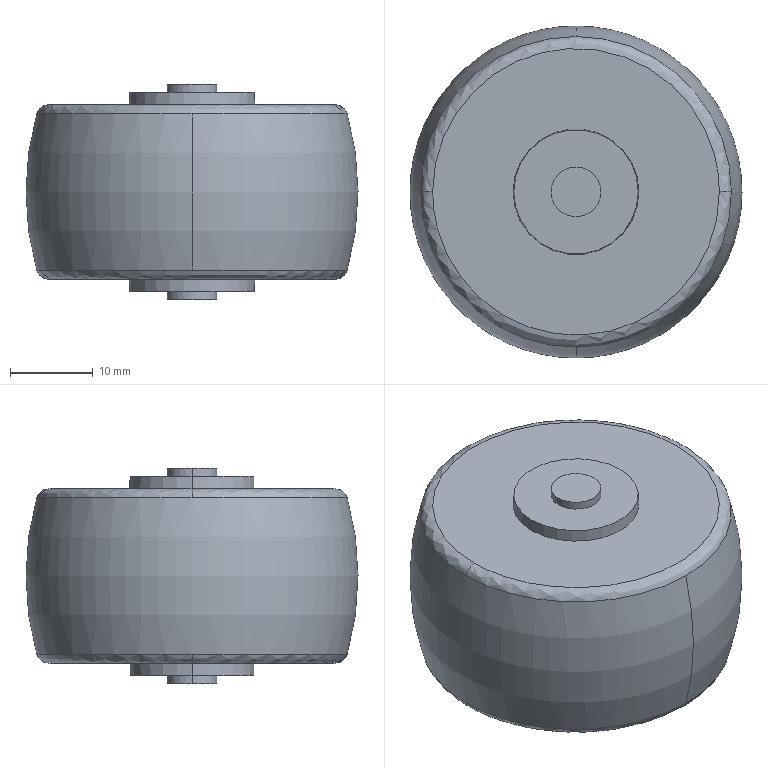Part | STEP file | _CMAZ40-N_w | 1 solid | 20 faces | box 40 x 40 x 26 mm | volume 25557 mm3 | plane 6 | spline 4 | cone 4 | cylinder 4 | torus 2 | commonest cylinder face diameters 6 x4
STEP:
#1=CARTESIAN_POINT('',(-17.268,0.,-10.5));
#2=VERTEX_POINT('',#1);
#3=CARTESIAN_POINT('',(17.268,0.,-10.5));
#4=VERTEX_POINT('',#3);
#5=CARTESIAN_POINT('',(-17.268,0.,-10.5));
#6=CARTESIAN_POINT('',(-17.268,-34.537,-10.5));
#7=CARTESIAN_POINT('',(17.268,-34.537,-10.5));
#8=CARTESIAN_POINT('',(17.268,0.,-10.5));
#9=(BOUNDED_CURVE()B_SPLINE_CURVE(3,(#5,#6,#7,#8),.UNSPECIFIED.,.F.,.T.)B_SPLINE_CURVE_WITH_KNOTS((4,4),(0.,0.5),.UNSPECIFIED.)CURVE()GEOMETRIC_REPRESENTATION_ITEM()RATIONAL_B_SPLINE_CURVE((1.,0.3333,0.3333,1.))REPRESENTATION_ITEM(''));
#10=EDGE_CURVE('',#2,#4,#9,.T.);
#11=ORIENTED_EDGE('',*,*,#10,.T.);
#12=CARTESIAN_POINT('',(18.713,0.,-9.403));
#13=VERTEX_POINT('',#12);
#14=CARTESIAN_POINT('',(17.268,0.,-9.));
#15=DIRECTION('',(0.,-1.,0.));
#16=DIRECTION('',(1.,0.,0.));
#17=AXIS2_PLACEMENT_3D('',#14,#15,#16);
#18=CIRCLE('',#17,1.5);
#19=EDGE_CURVE('',#4,#13,#18,.T.);
#20=ORIENTED_EDGE('',*,*,#19,.T.);
#21=CARTESIAN_POINT('',(0.,-18.713,-9.403));
#22=VERTEX_POINT('',#21);
#23=CARTESIAN_POINT('',(0.,0.,-9.403));
#24=DIRECTION('',(0.,0.,1.));
#25=DIRECTION('',(0.,-1.,0.));
#26=AXIS2_PLACEMENT_3D('',#23,#24,#25);
#27=CIRCLE('',#26,18.713);
#28=EDGE_CURVE('',#22,#13,#27,.T.);
#29=ORIENTED_EDGE('',*,*,#28,.F.);
#30=CARTESIAN_POINT('',(-18.713,0.,-9.403));
#31=VERTEX_POINT('',#30);
#32=CARTESIAN_POINT('',(0.,0.,-9.403));
#33=DIRECTION('',(0.,0.,1.));
#34=DIRECTION('',(0.,-1.,0.));
#35=AXIS2_PLACEMENT_3D('',#32,#33,#34);
#36=CIRCLE('',#35,18.713);
#37=EDGE_CURVE('',#31,#22,#36,.T.);
#38=ORIENTED_EDGE('',*,*,#37,.F.);
#39=CARTESIAN_POINT('',(-17.268,0.,-9.));
#40=DIRECTION('',(0.,1.,0.));
#41=DIRECTION('',(-1.,0.,0.));
#42=AXIS2_PLACEMENT_3D('',#39,#40,#41);
#43=CIRCLE('',#42,1.5);
#44=EDGE_CURVE('',#2,#31,#43,.T.);
#45=ORIENTED_EDGE('',*,*,#44,.F.);
#46=EDGE_LOOP('',(#11,#20,#29,#38,#45));
#47=FACE_OUTER_BOUND('',#46,.T.);
#48=CARTESIAN_POINT('',(17.268,0.,-10.5));
#49=CARTESIAN_POINT('',(17.268,-34.537,-10.5));
#50=CARTESIAN_POINT('',(-17.268,-34.537,-10.5));
#51=CARTESIAN_POINT('',(-17.268,0.,-10.5));
#52=CARTESIAN_POINT('',(17.968,0.,-10.5));
#53=CARTESIAN_POINT('',(17.968,-35.936,-10.5));
#54=CARTESIAN_POINT('',(-17.968,-35.936,-10.5));
#55=CARTESIAN_POINT('',(-17.968,0.,-10.5));
#56=CARTESIAN_POINT('',(18.525,0.,-10.077));
#57=CARTESIAN_POINT('',(18.525,-37.051,-10.077));
#58=CARTESIAN_POINT('',(-18.525,-37.051,-10.077));
#59=CARTESIAN_POINT('',(-18.525,0.,-10.077));
#60=CARTESIAN_POINT('',(18.713,0.,-9.403));
#61=CARTESIAN_POINT('',(18.713,-37.427,-9.403));
#62=CARTESIAN_POINT('',(-18.713,-37.427,-9.403));
#63=CARTESIAN_POINT('',(-18.713,0.,-9.403));
#64=(BOUNDED_SURFACE()B_SPLINE_SURFACE(3,3,((#48,#49,#50,#51),(#52,#53,#54,#55),(#56,#57,#58,#59),(#60,#61,#62,#63)),.UNSPECIFIED.,.F.,.F.,.T.)B_SPLINE_SURFACE_WITH_KNOTS((4,4),(4,4),(0.,1.),(0.,1.),.UNSPECIFIED.)GEOMETRIC_REPRESENTATION_ITEM()RATIONAL_B_SPLINE_SURFACE(((1.,0.3333,0.3333,1.),(0.8643,0.2881,0.2881,0.8643),(0.8643,0.2881,0.2881,0.8643),(1.,0.3333,0.3333,1.)))REPRESENTATION_ITEM('')SURFACE());
#65=ADVANCED_FACE('',(#47),#64,.T.);
#66=CARTESIAN_POINT('',(18.713,0.,9.403));
#67=VERTEX_POINT('',#66);
#68=CARTESIAN_POINT('',(0.,-18.713,9.403));
#69=VERTEX_POINT('',#68);
#70=CARTESIAN_POINT('',(0.,0.,9.403));
#71=DIRECTION('',(0.,0.,-1.));
#72=DIRECTION('',(-1.,0.,0.));
#73=AXIS2_PLACEMENT_3D('',#70,#71,#72);
#74=CIRCLE('',#73,18.713);
#75=EDGE_CURVE('',#67,#69,#74,.T.);
#76=ORIENTED_EDGE('',*,*,#75,.F.);
#77=CARTESIAN_POINT('',(17.268,0.,10.5));
#78=VERTEX_POINT('',#77);
#79=CARTESIAN_POINT('',(17.268,0.,9.));
#80=DIRECTION('',(0.,-1.,0.));
#81=DIRECTION('',(1.,0.,0.));
#82=AXIS2_PLACEMENT_3D('',#79,#80,#81);
#83=CIRCLE('',#82,1.5);
#84=EDGE_CURVE('',#67,#78,#83,.T.);
#85=ORIENTED_EDGE('',*,*,#84,.T.);
#86=CARTESIAN_POINT('',(-17.268,0.,10.5));
#87=VERTEX_POINT('',#86);
#88=CARTESIAN_POINT('',(17.268,0.,10.5));
#89=CARTESIAN_POINT('',(17.268,-34.537,10.5));
#90=CARTESIAN_POINT('',(-17.268,-34.537,10.5));
#91=CARTESIAN_POINT('',(-17.268,0.,10.5));
#92=(BOUNDED_CURVE()B_SPLINE_CURVE(3,(#88,#89,#90,#91),.UNSPECIFIED.,.F.,.F.)B_SPLINE_CURVE_WITH_KNOTS((4,4),(0.5,1.),.UNSPECIFIED.)CURVE()GEOMETRIC_REPRESENTATION_ITEM()RATIONAL_B_SPLINE_CURVE((1.,0.3333,0.3333,1.))REPRESENTATION_ITEM(''));
#93=EDGE_CURVE('',#78,#87,#92,.T.);
#94=ORIENTED_EDGE('',*,*,#93,.T.);
#95=CARTESIAN_POINT('',(-18.713,0.,9.403));
#96=VERTEX_POINT('',#95);
#97=CARTESIAN_POINT('',(-17.268,0.,9.));
#98=DIRECTION('',(0.,1.,0.));
#99=DIRECTION('',(-1.,0.,0.));
#100=AXIS2_PLACEMENT_3D('',#97,#98,#99);
#101=CIRCLE('',#100,1.5);
#102=EDGE_CURVE('',#96,#87,#101,.T.);
#103=ORIENTED_EDGE('',*,*,#102,.F.);
#104=CARTESIAN_POINT('',(0.,0.,9.403));
#105=DIRECTION('',(0.,0.,-1.));
#106=DIRECTION('',(-1.,0.,0.));
#107=AXIS2_PLACEMENT_3D('',#104,#105,#106);
#108=CIRCLE('',#107,18.713);
#109=EDGE_CURVE('',#69,#96,#108,.T.);
#110=ORIENTED_EDGE('',*,*,#109,.F.);
#111=EDGE_LOOP('',(#76,#85,#94,#103,#110));
#112=FACE_OUTER_BOUND('',#111,.T.);
#113=CARTESIAN_POINT('',(18.713,0.,9.403));
#114=CARTESIAN_POINT('',(18.713,-37.427,9.403));
#115=CARTESIAN_POINT('',(-18.713,-37.427,9.403));
#116=CARTESIAN_POINT('',(-18.713,0.,9.403));
#117=CARTESIAN_POINT('',(18.525,0.,10.077));
#118=CARTESIAN_POINT('',(18.525,-37.051,10.077));
#119=CARTESIAN_POINT('',(-18.525,-37.051,10.077));
#120=CARTESIAN_POINT('',(-18.525,0.,10.077));
#121=CARTESIAN_POINT('',(17.968,0.,10.5));
#122=CARTESIAN_POINT('',(17.968,-35.936,10.5));
#123=CARTESIAN_POINT('',(-17.968,-35.936,10.5));
#124=CARTESIAN_POINT('',(-17.968,0.,10.5));
#125=CARTESIAN_POINT('',(17.268,0.,10.5));
#126=CARTESIAN_POINT('',(17.268,-34.537,10.5));
#127=CARTESIAN_POINT('',(-17.268,-34.537,10.5));
#128=CARTESIAN_POINT('',(-17.268,0.,10.5));
#129=(BOUNDED_SURFACE()B_SPLINE_SURFACE(3,3,((#113,#114,#115,#116),(#117,#118,#119,#120),(#121,#122,#123,#124),(#125,#126,#127,#128)),.UNSPECIFIED.,.F.,.F.,.F.)B_SPLINE_SURFACE_WITH_KNOTS((4,4),(4,4),(0.,1.),(0.,1.),.UNSPECIFIED.)GEOMETRIC_REPRESENTATION_ITEM()RATIONAL_B_SPLINE_SURFACE(((1.,0.3333,0.3333,1.),(0.8643,0.2881,0.2881,0.8643),(0.8643,0.2881,0.2881,0.8643),(1.,0.3333,0.3333,1.)))REPRESENTATION_ITEM('')SURFACE());
#130=ADVANCED_FACE('',(#112),#129,.T.);
#131=CARTESIAN_POINT('',(0.,18.713,9.403));
#132=VERTEX_POINT('',#131);
#133=CARTESIAN_POINT('',(0.,0.,9.403));
#134=DIRECTION('',(0.,0.,-1.));
#135=DIRECTION('',(-1.,0.,0.));
#136=AXIS2_PLACEMENT_3D('',#133,#134,#135);
#137=CIRCLE('',#136,18.713);
#138=EDGE_CURVE('',#132,#67,#137,.T.);
#139=ORIENTED_EDGE('',*,*,#138,.T.);
#140=ORIENTED_EDGE('',*,*,#75,.T.);
#141=CARTESIAN_POINT('',(0.,15.,0.));
#142=DIRECTION('',(1.,0.,0.));
#143=DIRECTION('',(0.,1.,0.));
#144=AXIS2_PLACEMENT_3D('',#141,#142,#143);
#145=CIRCLE('',#144,35.);
#146=EDGE_CURVE('',#69,#22,#145,.T.);
#147=ORIENTED_EDGE('',*,*,#146,.T.);
#148=ORIENTED_EDGE('',*,*,#28,.T.);
#149=CARTESIAN_POINT('',(0.,18.713,-9.403));
#150=VERTEX_POINT('',#149);
#151=CARTESIAN_POINT('',(0.,0.,-9.403));
#152=DIRECTION('',(0.,0.,1.));
#153=DIRECTION('',(0.,-1.,0.));
#154=AXIS2_PLACEMENT_3D('',#151,#152,#153);
#155=CIRCLE('',#154,18.713);
#156=EDGE_CURVE('',#13,#150,#155,.T.);
#157=ORIENTED_EDGE('',*,*,#156,.T.);
#158=CARTESIAN_POINT('',(0.,-15.,0.));
#159=DIRECTION('',(-1.,0.,0.));
#160=DIRECTION('',(0.,0.,1.));
#161=AXIS2_PLACEMENT_3D('',#158,#159,#160);
#162=CIRCLE('',#161,35.);
#163=EDGE_CURVE('',#132,#150,#162,.T.);
#164=ORIENTED_EDGE('',*,*,#163,.F.);
#165=EDGE_LOOP('',(#139,#140,#147,#148,#157,#164));
#166=FACE_OUTER_BOUND('',#165,.T.);
#167=CARTESIAN_POINT('',(0.,0.,0.));
#168=DIRECTION('',(0.,0.,-1.));
#169=DIRECTION('',(0.,1.,0.));
#170=AXIS2_PLACEMENT_3D('',#167,#168,#169);
#171=TOROIDAL_SURFACE('',#170,-15.,35.);
#172=ADVANCED_FACE('',(#166),#171,.T.);
#173=CARTESIAN_POINT('',(7.5,0.,-12.));
#174=VERTEX_POINT('',#173);
#175=CARTESIAN_POINT('',(-7.5,0.,-12.));
#176=VERTEX_POINT('',#175);
#177=CARTESIAN_POINT('',(0.,0.,-12.));
#178=DIRECTION('',(0.,0.,1.));
#179=DIRECTION('',(1.,0.,0.));
#180=AXIS2_PLACEMENT_3D('',#177,#178,#179);
#181=CIRCLE('',#180,7.5);
#182=EDGE_CURVE('',#174,#176,#181,.T.);
#183=ORIENTED_EDGE('',*,*,#182,.T.);
#184=CARTESIAN_POINT('',(-7.579,0.,-10.5));
#185=VERTEX_POINT('',#184);
#186=CARTESIAN_POINT('',(-7.579,0.,-10.5));
#187=DIRECTION('',(-0.05226,0.,0.9986));
#188=VECTOR('',#187,1000.);
#189=LINE('',#186,#188);
#190=EDGE_CURVE('',#176,#185,#189,.T.);
#191=ORIENTED_EDGE('',*,*,#190,.T.);
#192=CARTESIAN_POINT('',(7.579,0.,-10.5));
#193=VERTEX_POINT('',#192);
#194=CARTESIAN_POINT('',(0.,0.,-10.5));
#195=DIRECTION('',(0.,0.,-1.));
#196=DIRECTION('',(1.,0.,0.));
#197=AXIS2_PLACEMENT_3D('',#194,#195,#196);
#198=CIRCLE('',#197,7.579);
#199=EDGE_CURVE('',#185,#193,#198,.T.);
#200=ORIENTED_EDGE('',*,*,#199,.T.);
#201=CARTESIAN_POINT('',(7.579,0.,-10.5));
#202=DIRECTION('',(0.05226,0.,0.9986));
#203=VECTOR('',#202,1000.);
#204=LINE('',#201,#203);
#205=EDGE_CURVE('',#174,#193,#204,.T.);
#206=ORIENTED_EDGE('',*,*,#205,.F.);
#207=EDGE_LOOP('',(#183,#191,#200,#206));
#208=FACE_OUTER_BOUND('',#207,.T.);
#209=CARTESIAN_POINT('',(0.,0.,-10.5));
#210=DIRECTION('',(0.,0.,1.));
#211=DIRECTION('',(1.,0.,0.));
#212=AXIS2_PLACEMENT_3D('',#209,#210,#211);
#213=CONICAL_SURFACE('',#212,7.579,0.05229);
#214=ADVANCED_FACE('',(#208),#213,.T.);
#215=CARTESIAN_POINT('',(-7.5,0.,12.));
#216=VERTEX_POINT('',#215);
#217=CARTESIAN_POINT('',(7.5,0.,12.));
#218=VERTEX_POINT('',#217);
#219=CARTESIAN_POINT('',(0.,0.,12.));
#220=DIRECTION('',(0.,0.,-1.));
#221=DIRECTION('',(-1.,0.,0.));
#222=AXIS2_PLACEMENT_3D('',#219,#220,#221);
#223=CIRCLE('',#222,7.5);
#224=EDGE_CURVE('',#216,#218,#223,.T.);
#225=ORIENTED_EDGE('',*,*,#224,.T.);
#226=CARTESIAN_POINT('',(7.579,0.,10.5));
#227=VERTEX_POINT('',#226);
#228=CARTESIAN_POINT('',(7.579,0.,10.5));
#229=DIRECTION('',(0.05226,0.,-0.9986));
#230=VECTOR('',#229,1000.);
#231=LINE('',#228,#230);
#232=EDGE_CURVE('',#218,#227,#231,.T.);
#233=ORIENTED_EDGE('',*,*,#232,.T.);
#234=CARTESIAN_POINT('',(-7.579,0.,10.5));
#235=VERTEX_POINT('',#234);
#236=CARTESIAN_POINT('',(0.,0.,10.5));
#237=DIRECTION('',(0.,0.,1.));
#238=DIRECTION('',(-1.,0.,0.));
#239=AXIS2_PLACEMENT_3D('',#236,#237,#238);
#240=CIRCLE('',#239,7.579);
#241=EDGE_CURVE('',#227,#235,#240,.T.);
#242=ORIENTED_EDGE('',*,*,#241,.T.);
#243=CARTESIAN_POINT('',(-7.579,0.,10.5));
#244=DIRECTION('',(-0.05226,0.,-0.9986));
#245=VECTOR('',#244,1000.);
#246=LINE('',#243,#245);
#247=EDGE_CURVE('',#216,#235,#246,.T.);
#248=ORIENTED_EDGE('',*,*,#247,.F.);
#249=EDGE_LOOP('',(#225,#233,#242,#248));
#250=FACE_OUTER_BOUND('',#249,.T.);
#251=CARTESIAN_POINT('',(0.,0.,10.5));
#252=DIRECTION('',(0.,0.,-1.));
#253=DIRECTION('',(-1.,0.,0.));
#254=AXIS2_PLACEMENT_3D('',#251,#252,#253);
#255=CONICAL_SURFACE('',#254,7.579,0.05229);
#256=ADVANCED_FACE('',(#250),#255,.T.);
#257=CARTESIAN_POINT('',(3.,0.,-13.));
#258=VERTEX_POINT('',#257);
#259=CARTESIAN_POINT('',(-3.,0.,-13.));
#260=VERTEX_POINT('',#259);
#261=CARTESIAN_POINT('',(0.,0.,-13.));
#262=DIRECTION('',(0.,0.,1.));
#263=DIRECTION('',(1.,0.,0.));
#264=AXIS2_PLACEMENT_3D('',#261,#262,#263);
#265=CIRCLE('',#264,3.);
#266=EDGE_CURVE('',#258,#260,#265,.T.);
#267=ORIENTED_EDGE('',*,*,#266,.T.);
#268=CARTESIAN_POINT('',(-3.,0.,-12.));
#269=VERTEX_POINT('',#268);
#270=CARTESIAN_POINT('',(-3.,0.,-13.));
#271=DIRECTION('',(0.,0.,1.));
#272=VECTOR('',#271,1000.);
#273=LINE('',#270,#272);
#274=EDGE_CURVE('',#260,#269,#273,.T.);
#275=ORIENTED_EDGE('',*,*,#274,.T.);
#276=CARTESIAN_POINT('',(3.,0.,-12.));
#277=VERTEX_POINT('',#276);
#278=CARTESIAN_POINT('',(0.,0.,-12.));
#279=DIRECTION('',(0.,0.,-1.));
#280=DIRECTION('',(1.,0.,0.));
#281=AXIS2_PLACEMENT_3D('',#278,#279,#280);
#282=CIRCLE('',#281,3.);
#283=EDGE_CURVE('',#269,#277,#282,.T.);
#284=ORIENTED_EDGE('',*,*,#283,.T.);
#285=CARTESIAN_POINT('',(3.,0.,-13.));
#286=DIRECTION('',(0.,0.,1.));
#287=VECTOR('',#286,1000.);
#288=LINE('',#285,#287);
#289=EDGE_CURVE('',#258,#277,#288,.T.);
#290=ORIENTED_EDGE('',*,*,#289,.F.);
#291=EDGE_LOOP('',(#267,#275,#284,#290));
#292=FACE_OUTER_BOUND('',#291,.T.);
#293=CARTESIAN_POINT('',(0.,0.,-13.));
#294=DIRECTION('',(0.,0.,1.));
#295=DIRECTION('',(1.,0.,0.));
#296=AXIS2_PLACEMENT_3D('',#293,#294,#295);
#297=CYLINDRICAL_SURFACE('',#296,3.);
#298=ADVANCED_FACE('',(#292),#297,.T.);
#299=CARTESIAN_POINT('',(3.,0.,12.));
#300=VERTEX_POINT('',#299);
#301=CARTESIAN_POINT('',(-3.,0.,12.));
#302=VERTEX_POINT('',#301);
#303=CARTESIAN_POINT('',(0.,0.,12.));
#304=DIRECTION('',(0.,0.,1.));
#305=DIRECTION('',(1.,0.,0.));
#306=AXIS2_PLACEMENT_3D('',#303,#304,#305);
#307=CIRCLE('',#306,3.);
#308=EDGE_CURVE('',#300,#302,#307,.T.);
#309=ORIENTED_EDGE('',*,*,#308,.T.);
#310=CARTESIAN_POINT('',(-3.,0.,13.));
#311=VERTEX_POINT('',#310);
#312=CARTESIAN_POINT('',(-3.,0.,-13.));
#313=DIRECTION('',(0.,0.,1.));
#314=VECTOR('',#313,1000.);
#315=LINE('',#312,#314);
#316=EDGE_CURVE('',#302,#311,#315,.T.);
#317=ORIENTED_EDGE('',*,*,#316,.T.);
#318=CARTESIAN_POINT('',(3.,0.,13.));
#319=VERTEX_POINT('',#318);
#320=CARTESIAN_POINT('',(0.,0.,13.));
#321=DIRECTION('',(0.,0.,-1.));
#322=DIRECTION('',(1.,0.,0.));
#323=AXIS2_PLACEMENT_3D('',#320,#321,#322);
#324=CIRCLE('',#323,3.);
#325=EDGE_CURVE('',#311,#319,#324,.T.);
#326=ORIENTED_EDGE('',*,*,#325,.T.);
#327=CARTESIAN_POINT('',(3.,0.,-13.));
#328=DIRECTION('',(0.,0.,1.));
#329=VECTOR('',#328,1000.);
#330=LINE('',#327,#329);
#331=EDGE_CURVE('',#300,#319,#330,.T.);
#332=ORIENTED_EDGE('',*,*,#331,.F.);
#333=EDGE_LOOP('',(#309,#317,#326,#332));
#334=FACE_OUTER_BOUND('',#333,.T.);
#335=CARTESIAN_POINT('',(0.,0.,-13.));
#336=DIRECTION('',(0.,0.,1.));
#337=DIRECTION('',(1.,0.,0.));
#338=AXIS2_PLACEMENT_3D('',#335,#336,#337);
#339=CYLINDRICAL_SURFACE('',#338,3.);
#340=ADVANCED_FACE('',(#334),#339,.T.);
#341=ORIENTED_EDGE('',*,*,#146,.F.);
#342=ORIENTED_EDGE('',*,*,#109,.T.);
#343=CARTESIAN_POINT('',(0.,0.,9.403));
#344=DIRECTION('',(0.,0.,-1.));
#345=DIRECTION('',(-1.,0.,0.));
#346=AXIS2_PLACEMENT_3D('',#343,#344,#345);
#347=CIRCLE('',#346,18.713);
#348=EDGE_CURVE('',#96,#132,#347,.T.);
#349=ORIENTED_EDGE('',*,*,#348,.T.);
#350=ORIENTED_EDGE('',*,*,#163,.T.);
#351=CARTESIAN_POINT('',(0.,0.,-9.403));
#352=DIRECTION('',(0.,0.,1.));
#353=DIRECTION('',(0.,-1.,0.));
#354=AXIS2_PLACEMENT_3D('',#351,#352,#353);
#355=CIRCLE('',#354,18.713);
#356=EDGE_CURVE('',#150,#31,#355,.T.);
#357=ORIENTED_EDGE('',*,*,#356,.T.);
#358=ORIENTED_EDGE('',*,*,#37,.T.);
#359=EDGE_LOOP('',(#341,#342,#349,#350,#357,#358));
#360=FACE_OUTER_BOUND('',#359,.T.);
#361=CARTESIAN_POINT('',(0.,0.,0.));
#362=DIRECTION('',(0.,0.,-1.));
#363=DIRECTION('',(0.,1.,0.));
#364=AXIS2_PLACEMENT_3D('',#361,#362,#363);
#365=TOROIDAL_SURFACE('',#364,-15.,35.);
#366=ADVANCED_FACE('',(#360),#365,.T.);
#367=ORIENTED_EDGE('',*,*,#19,.F.);
#368=CARTESIAN_POINT('',(17.268,0.,-10.5));
#369=CARTESIAN_POINT('',(17.268,34.537,-10.5));
#370=CARTESIAN_POINT('',(-17.268,34.537,-10.5));
#371=CARTESIAN_POINT('',(-17.268,0.,-10.5));
#372=(BOUNDED_CURVE()B_SPLINE_CURVE(3,(#368,#369,#370,#371),.UNSPECIFIED.,.F.,.T.)B_SPLINE_CURVE_WITH_KNOTS((4,4),(0.5,1.),.UNSPECIFIED.)CURVE()GEOMETRIC_REPRESENTATION_ITEM()RATIONAL_B_SPLINE_CURVE((1.,0.3333,0.3333,1.))REPRESENTATION_ITEM(''));
#373=EDGE_CURVE('',#4,#2,#372,.T.);
#374=ORIENTED_EDGE('',*,*,#373,.T.);
#375=ORIENTED_EDGE('',*,*,#44,.T.);
#376=ORIENTED_EDGE('',*,*,#356,.F.);
#377=ORIENTED_EDGE('',*,*,#156,.F.);
#378=EDGE_LOOP('',(#367,#374,#375,#376,#377));
#379=FACE_OUTER_BOUND('',#378,.T.);
#380=CARTESIAN_POINT('',(-17.268,0.,-10.5));
#381=CARTESIAN_POINT('',(-17.268,34.537,-10.5));
#382=CARTESIAN_POINT('',(17.268,34.537,-10.5));
#383=CARTESIAN_POINT('',(17.268,0.,-10.5));
#384=CARTESIAN_POINT('',(-17.968,0.,-10.5));
#385=CARTESIAN_POINT('',(-17.968,35.936,-10.5));
#386=CARTESIAN_POINT('',(17.968,35.936,-10.5));
#387=CARTESIAN_POINT('',(17.968,0.,-10.5));
#388=CARTESIAN_POINT('',(-18.525,0.,-10.077));
#389=CARTESIAN_POINT('',(-18.525,37.051,-10.077));
#390=CARTESIAN_POINT('',(18.525,37.051,-10.077));
#391=CARTESIAN_POINT('',(18.525,0.,-10.077));
#392=CARTESIAN_POINT('',(-18.713,0.,-9.403));
#393=CARTESIAN_POINT('',(-18.713,37.427,-9.403));
#394=CARTESIAN_POINT('',(18.713,37.427,-9.403));
#395=CARTESIAN_POINT('',(18.713,0.,-9.403));
#396=(BOUNDED_SURFACE()B_SPLINE_SURFACE(3,3,((#380,#381,#382,#383),(#384,#385,#386,#387),(#388,#389,#390,#391),(#392,#393,#394,#395)),.UNSPECIFIED.,.F.,.F.,.F.)B_SPLINE_SURFACE_WITH_KNOTS((4,4),(4,4),(0.,1.),(0.,1.),.UNSPECIFIED.)GEOMETRIC_REPRESENTATION_ITEM()RATIONAL_B_SPLINE_SURFACE(((1.,0.3333,0.3333,1.),(0.8643,0.2881,0.2881,0.8643),(0.8643,0.2881,0.2881,0.8643),(1.,0.3333,0.3333,1.)))REPRESENTATION_ITEM('')SURFACE());
#397=ADVANCED_FACE('',(#379),#396,.T.);
#398=ORIENTED_EDGE('',*,*,#84,.F.);
#399=ORIENTED_EDGE('',*,*,#138,.F.);
#400=ORIENTED_EDGE('',*,*,#348,.F.);
#401=ORIENTED_EDGE('',*,*,#102,.T.);
#402=CARTESIAN_POINT('',(-17.268,0.,10.5));
#403=CARTESIAN_POINT('',(-17.268,34.537,10.5));
#404=CARTESIAN_POINT('',(17.268,34.537,10.5));
#405=CARTESIAN_POINT('',(17.268,0.,10.5));
#406=(BOUNDED_CURVE()B_SPLINE_CURVE(3,(#402,#403,#404,#405),.UNSPECIFIED.,.F.,.T.)B_SPLINE_CURVE_WITH_KNOTS((4,4),(0.,0.5),.UNSPECIFIED.)CURVE()GEOMETRIC_REPRESENTATION_ITEM()RATIONAL_B_SPLINE_CURVE((1.,0.3333,0.3333,1.))REPRESENTATION_ITEM(''));
#407=EDGE_CURVE('',#87,#78,#406,.T.);
#408=ORIENTED_EDGE('',*,*,#407,.T.);
#409=EDGE_LOOP('',(#398,#399,#400,#401,#408));
#410=FACE_OUTER_BOUND('',#409,.T.);
#411=CARTESIAN_POINT('',(-18.713,0.,9.403));
#412=CARTESIAN_POINT('',(-18.713,37.427,9.403));
#413=CARTESIAN_POINT('',(18.713,37.427,9.403));
#414=CARTESIAN_POINT('',(18.713,0.,9.403));
#415=CARTESIAN_POINT('',(-18.525,0.,10.077));
#416=CARTESIAN_POINT('',(-18.525,37.051,10.077));
#417=CARTESIAN_POINT('',(18.525,37.051,10.077));
#418=CARTESIAN_POINT('',(18.525,0.,10.077));
#419=CARTESIAN_POINT('',(-17.968,0.,10.5));
#420=CARTESIAN_POINT('',(-17.968,35.936,10.5));
#421=CARTESIAN_POINT('',(17.968,35.936,10.5));
#422=CARTESIAN_POINT('',(17.968,0.,10.5));
#423=CARTESIAN_POINT('',(-17.268,0.,10.5));
#424=CARTESIAN_POINT('',(-17.268,34.537,10.5));
#425=CARTESIAN_POINT('',(17.268,34.537,10.5));
#426=CARTESIAN_POINT('',(17.268,0.,10.5));
#427=(BOUNDED_SURFACE()B_SPLINE_SURFACE(3,3,((#411,#412,#413,#414),(#415,#416,#417,#418),(#419,#420,#421,#422),(#423,#424,#425,#426)),.UNSPECIFIED.,.F.,.F.,.F.)B_SPLINE_SURFACE_WITH_KNOTS((4,4),(4,4),(0.,1.),(0.,1.),.UNSPECIFIED.)GEOMETRIC_REPRESENTATION_ITEM()RATIONAL_B_SPLINE_SURFACE(((1.,0.3333,0.3333,1.),(0.8643,0.2881,0.2881,0.8643),(0.8643,0.2881,0.2881,0.8643),(1.,0.3333,0.3333,1.)))REPRESENTATION_ITEM('')SURFACE());
#428=ADVANCED_FACE('',(#410),#427,.T.);
#429=ORIENTED_EDGE('',*,*,#10,.F.);
#430=ORIENTED_EDGE('',*,*,#373,.F.);
#431=EDGE_LOOP('',(#429,#430));
#432=FACE_OUTER_BOUND('',#431,.T.);
#433=CARTESIAN_POINT('',(0.,0.,-10.5));
#434=DIRECTION('',(0.,0.,-1.));
#435=DIRECTION('',(1.,0.,0.));
#436=AXIS2_PLACEMENT_3D('',#433,#434,#435);
#437=CIRCLE('',#436,7.579);
#438=EDGE_CURVE('',#193,#185,#437,.T.);
#439=ORIENTED_EDGE('',*,*,#438,.F.);
#440=ORIENTED_EDGE('',*,*,#199,.F.);
#441=EDGE_LOOP('',(#439,#440));
#442=FACE_BOUND('',#441,.T.);
#443=CARTESIAN_POINT('',(0.,17.268,-10.5));
#444=DIRECTION('',(0.,0.,1.));
#445=DIRECTION('',(1.,0.,0.));
#446=AXIS2_PLACEMENT_3D('',#443,#444,#445);
#447=PLANE('',#446);
#448=ADVANCED_FACE('',(#432,#442),#447,.F.);
#449=CARTESIAN_POINT('',(0.,0.,10.5));
#450=DIRECTION('',(0.,0.,1.));
#451=DIRECTION('',(-1.,0.,0.));
#452=AXIS2_PLACEMENT_3D('',#449,#450,#451);
#453=CIRCLE('',#452,7.579);
#454=EDGE_CURVE('',#235,#227,#453,.T.);
#455=ORIENTED_EDGE('',*,*,#454,.F.);
#456=ORIENTED_EDGE('',*,*,#241,.F.);
#457=EDGE_LOOP('',(#455,#456));
#458=FACE_BOUND('',#457,.T.);
#459=ORIENTED_EDGE('',*,*,#407,.F.);
#460=ORIENTED_EDGE('',*,*,#93,.F.);
#461=EDGE_LOOP('',(#459,#460));
#462=FACE_OUTER_BOUND('',#461,.T.);
#463=CARTESIAN_POINT('',(0.,7.579,10.5));
#464=DIRECTION('',(0.,0.,-1.));
#465=DIRECTION('',(-1.,0.,0.));
#466=AXIS2_PLACEMENT_3D('',#463,#464,#465);
#467=PLANE('',#466);
#468=ADVANCED_FACE('',(#458,#462),#467,.F.);
#469=ORIENTED_EDGE('',*,*,#190,.F.);
#470=CARTESIAN_POINT('',(0.,0.,-12.));
#471=DIRECTION('',(0.,0.,1.));
#472=DIRECTION('',(1.,0.,0.));
#473=AXIS2_PLACEMENT_3D('',#470,#471,#472);
#474=CIRCLE('',#473,7.5);
#475=EDGE_CURVE('',#176,#174,#474,.T.);
#476=ORIENTED_EDGE('',*,*,#475,.T.);
#477=ORIENTED_EDGE('',*,*,#205,.T.);
#478=ORIENTED_EDGE('',*,*,#438,.T.);
#479=EDGE_LOOP('',(#469,#476,#477,#478));
#480=FACE_OUTER_BOUND('',#479,.T.);
#481=CARTESIAN_POINT('',(0.,0.,-10.5));
#482=DIRECTION('',(0.,0.,1.));
#483=DIRECTION('',(1.,0.,0.));
#484=AXIS2_PLACEMENT_3D('',#481,#482,#483);
#485=CONICAL_SURFACE('',#484,7.579,0.05229);
#486=ADVANCED_FACE('',(#480),#485,.T.);
#487=ORIENTED_EDGE('',*,*,#232,.F.);
#488=CARTESIAN_POINT('',(0.,0.,12.));
#489=DIRECTION('',(0.,0.,-1.));
#490=DIRECTION('',(-1.,0.,0.));
#491=AXIS2_PLACEMENT_3D('',#488,#489,#490);
#492=CIRCLE('',#491,7.5);
#493=EDGE_CURVE('',#218,#216,#492,.T.);
#494=ORIENTED_EDGE('',*,*,#493,.T.);
#495=ORIENTED_EDGE('',*,*,#247,.T.);
#496=ORIENTED_EDGE('',*,*,#454,.T.);
#497=EDGE_LOOP('',(#487,#494,#495,#496));
#498=FACE_OUTER_BOUND('',#497,.T.);
#499=CARTESIAN_POINT('',(0.,0.,10.5));
#500=DIRECTION('',(0.,0.,-1.));
#501=DIRECTION('',(-1.,0.,0.));
#502=AXIS2_PLACEMENT_3D('',#499,#500,#501);
#503=CONICAL_SURFACE('',#502,7.579,0.05229);
#504=ADVANCED_FACE('',(#498),#503,.T.);
#505=ORIENTED_EDGE('',*,*,#182,.F.);
#506=ORIENTED_EDGE('',*,*,#475,.F.);
#507=EDGE_LOOP('',(#505,#506));
#508=FACE_OUTER_BOUND('',#507,.T.);
#509=CARTESIAN_POINT('',(0.,0.,-12.));
#510=DIRECTION('',(0.,0.,-1.));
#511=DIRECTION('',(1.,0.,0.));
#512=AXIS2_PLACEMENT_3D('',#509,#510,#511);
#513=CIRCLE('',#512,3.);
#514=EDGE_CURVE('',#277,#269,#513,.T.);
#515=ORIENTED_EDGE('',*,*,#514,.F.);
#516=ORIENTED_EDGE('',*,*,#283,.F.);
#517=EDGE_LOOP('',(#515,#516));
#518=FACE_BOUND('',#517,.T.);
#519=CARTESIAN_POINT('',(0.,7.5,-12.));
#520=DIRECTION('',(0.,0.,1.));
#521=DIRECTION('',(1.,0.,0.));
#522=AXIS2_PLACEMENT_3D('',#519,#520,#521);
#523=PLANE('',#522);
#524=ADVANCED_FACE('',(#508,#518),#523,.F.);
#525=ORIENTED_EDGE('',*,*,#308,.F.);
#526=CARTESIAN_POINT('',(0.,0.,12.));
#527=DIRECTION('',(0.,0.,1.));
#528=DIRECTION('',(1.,0.,0.));
#529=AXIS2_PLACEMENT_3D('',#526,#527,#528);
#530=CIRCLE('',#529,3.);
#531=EDGE_CURVE('',#302,#300,#530,.T.);
#532=ORIENTED_EDGE('',*,*,#531,.F.);
#533=EDGE_LOOP('',(#525,#532));
#534=FACE_BOUND('',#533,.T.);
#535=ORIENTED_EDGE('',*,*,#224,.F.);
#536=ORIENTED_EDGE('',*,*,#493,.F.);
#537=EDGE_LOOP('',(#535,#536));
#538=FACE_OUTER_BOUND('',#537,.T.);
#539=CARTESIAN_POINT('',(0.,3.,12.));
#540=DIRECTION('',(0.,0.,-1.));
#541=DIRECTION('',(-1.,0.,0.));
#542=AXIS2_PLACEMENT_3D('',#539,#540,#541);
#543=PLANE('',#542);
#544=ADVANCED_FACE('',(#534,#538),#543,.F.);
#545=ORIENTED_EDGE('',*,*,#274,.F.);
#546=CARTESIAN_POINT('',(0.,0.,-13.));
#547=DIRECTION('',(0.,0.,1.));
#548=DIRECTION('',(1.,0.,0.));
#549=AXIS2_PLACEMENT_3D('',#546,#547,#548);
#550=CIRCLE('',#549,3.);
#551=EDGE_CURVE('',#260,#258,#550,.T.);
#552=ORIENTED_EDGE('',*,*,#551,.T.);
#553=ORIENTED_EDGE('',*,*,#289,.T.);
#554=ORIENTED_EDGE('',*,*,#514,.T.);
#555=EDGE_LOOP('',(#545,#552,#553,#554));
#556=FACE_OUTER_BOUND('',#555,.T.);
#557=CARTESIAN_POINT('',(0.,0.,-13.));
#558=DIRECTION('',(0.,0.,1.));
#559=DIRECTION('',(1.,0.,0.));
#560=AXIS2_PLACEMENT_3D('',#557,#558,#559);
#561=CYLINDRICAL_SURFACE('',#560,3.);
#562=ADVANCED_FACE('',(#556),#561,.T.);
#563=ORIENTED_EDGE('',*,*,#316,.F.);
#564=ORIENTED_EDGE('',*,*,#531,.T.);
#565=ORIENTED_EDGE('',*,*,#331,.T.);
#566=CARTESIAN_POINT('',(0.,0.,13.));
#567=DIRECTION('',(0.,0.,-1.));
#568=DIRECTION('',(1.,0.,0.));
#569=AXIS2_PLACEMENT_3D('',#566,#567,#568);
#570=CIRCLE('',#569,3.);
#571=EDGE_CURVE('',#319,#311,#570,.T.);
#572=ORIENTED_EDGE('',*,*,#571,.T.);
#573=EDGE_LOOP('',(#563,#564,#565,#572));
#574=FACE_OUTER_BOUND('',#573,.T.);
#575=CARTESIAN_POINT('',(0.,0.,-13.));
#576=DIRECTION('',(0.,0.,1.));
#577=DIRECTION('',(1.,0.,0.));
#578=AXIS2_PLACEMENT_3D('',#575,#576,#577);
#579=CYLINDRICAL_SURFACE('',#578,3.);
#580=ADVANCED_FACE('',(#574),#579,.T.);
#581=ORIENTED_EDGE('',*,*,#266,.F.);
#582=ORIENTED_EDGE('',*,*,#551,.F.);
#583=EDGE_LOOP('',(#581,#582));
#584=FACE_OUTER_BOUND('',#583,.T.);
#585=CARTESIAN_POINT('',(0.,3.,-13.));
#586=DIRECTION('',(0.,0.,1.));
#587=DIRECTION('',(1.,0.,0.));
#588=AXIS2_PLACEMENT_3D('',#585,#586,#587);
#589=PLANE('',#588);
#590=ADVANCED_FACE('',(#584),#589,.F.);
#591=ORIENTED_EDGE('',*,*,#571,.F.);
#592=ORIENTED_EDGE('',*,*,#325,.F.);
#593=EDGE_LOOP('',(#591,#592));
#594=FACE_OUTER_BOUND('',#593,.T.);
#595=CARTESIAN_POINT('',(0.,0.,13.));
#596=DIRECTION('',(0.,0.,-1.));
#597=DIRECTION('',(-1.,0.,0.));
#598=AXIS2_PLACEMENT_3D('',#595,#596,#597);
#599=PLANE('',#598);
#600=ADVANCED_FACE('',(#594),#599,.F.);
#601=CLOSED_SHELL('',(#65,#130,#172,#214,#256,#298,#340,#366,#397,#428,#448,#468,#486,#504,#524,#544,#562,#580,#590,#600));
#602=MANIFOLD_SOLID_BREP('',#601);
#603=CARTESIAN_POINT('',(0.,0.,0.));
#604=DIRECTION('',(0.,0.,1.));
#605=DIRECTION('',(1.,0.,0.));
#606=AXIS2_PLACEMENT_3D('',#603,#604,#605);
#607=(LENGTH_UNIT()NAMED_UNIT(*)SI_UNIT(.MILLI.,.METRE.));
#608=UNCERTAINTY_MEASURE_WITH_UNIT(LENGTH_MEASURE(0.00001),#607,'','');
#609=(NAMED_UNIT(*)PLANE_ANGLE_UNIT()SI_UNIT($,.RADIAN.));
#610=(NAMED_UNIT(*)SI_UNIT($,.STERADIAN.)SOLID_ANGLE_UNIT());
#611=(GEOMETRIC_REPRESENTATION_CONTEXT(3)GLOBAL_UNCERTAINTY_ASSIGNED_CONTEXT((#608))GLOBAL_UNIT_ASSIGNED_CONTEXT((#607,#609,#610))REPRESENTATION_CONTEXT('',''));
#612=ADVANCED_BREP_SHAPE_REPRESENTATION('',(#602,#606),#611);